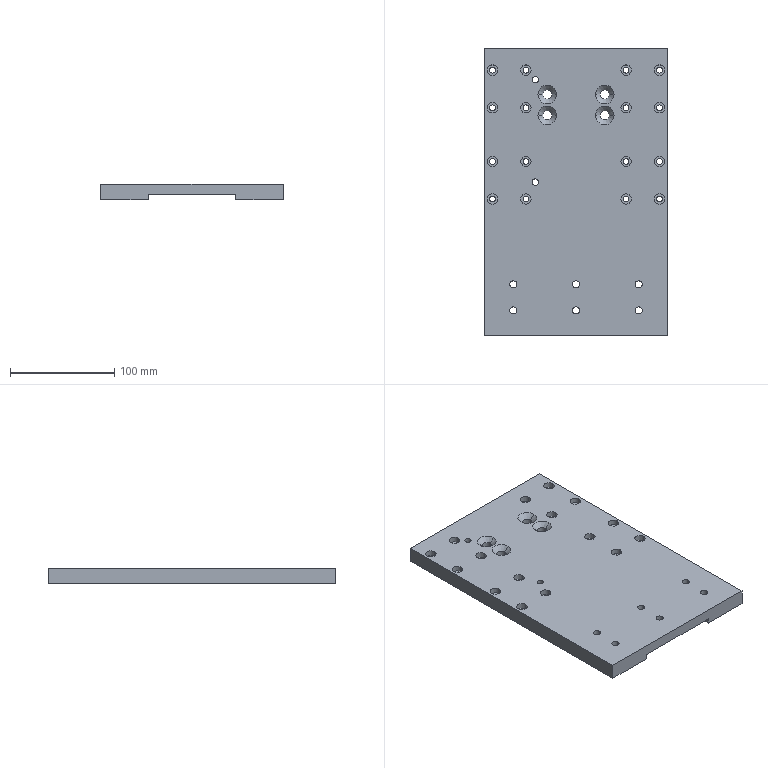Part | SolidWorks | features HoleWzd 4, Extrusion 1, ICE 1 | 1 solid | 122 faces | box 175 x 275 x 15 mm | volume 588428 mm3 | cylinder 88 | plane 26 | cone 8 | commonest cylinder face diameters 5.5 x32 10 x32 6.8 x12 9 x8 6 x4